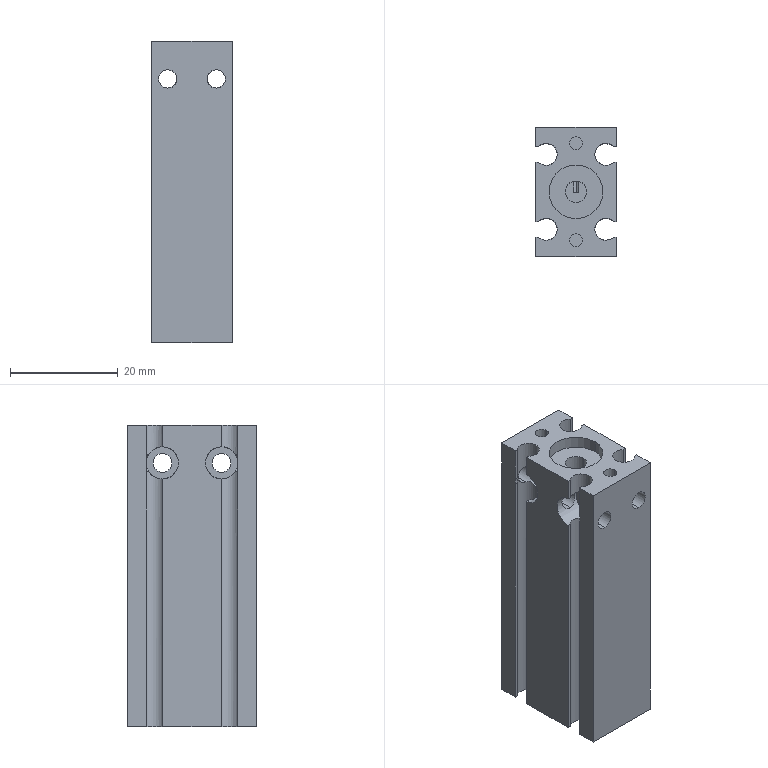Part | SolidWorks | features BaseBody 1 | 1 solid | 112 faces | box 15 x 24 x 56 mm | volume 13473 mm3 | cylinder 62 | plane 42 | cone 8 | commonest cylinder face diameters 3.4 x12 6 x12 2.459 x8 4.1 x8 10 x6 1 x4